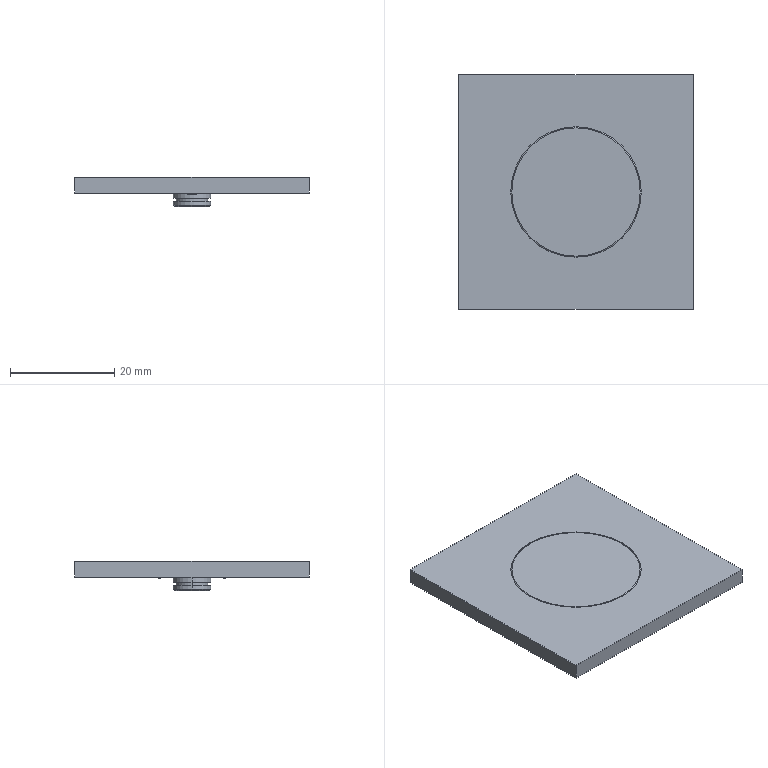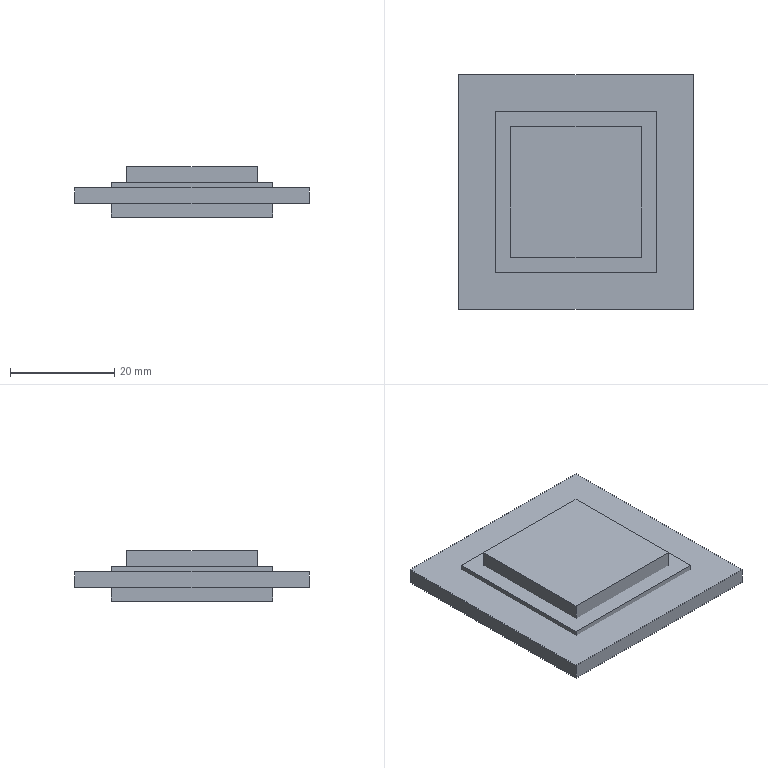CAM job | NX | 3-axis milling | part box 45 x 45 x 5.6 mm | stock box 45 x 45 x 9.6 mm
Tools:
number,name,description,diameter,corner_radius,flute_length,length,flutes
1,D6A45,Milling Tool-5 Parameters,6.0,0.0,50.0,75.0,2
14,D10JING,Milling Tool-5 Parameters,10.0,0.0,50.0,75.0,2
17,D4,Milling Tool-5 Parameters,4.0,0.0,50.0,75.0,2
18,D2,Milling Tool-5 Parameters,2.0,0.0,50.0,75.0,2
12,D2R0.5,Milling Tool-5 Parameters,2.0,0.5,50.0,75.0,2
24,T8H0.6,Milling Tool-T Cutter,8.0,,0.6,25.0,4
Operations:
program,operation,operation_type,tool,method,geometry_group,spindle_rpm,surface_speed,feed_per_tooth,feed_cut,feed_plunge,cut_length_mm,path_length_mm,cut_time_min,machine_time_min
1,FLOOR_WALL,VolumeBased25DMillingOperation,D10JING,METHOD,A,9500.0,298.0,0.0658,1250.0,100.0,325.997,379.997,0.2608,0.2662
1,PLANAR_MILL,PlanarMilling,D6A45,METHOD,A,9500.0,179.0,0.0658,1250.0,100.0,90.155,149.155,0.0721,0.078
1,ZLEVEL_PROFILE,ZLevelMilling,D10JING,METHOD,A,9500.0,298.0,0.1316,2500.0,100.0,765.005,827.605,0.306,0.3123
1,ZLEVEL_PROFILE_COPY_1,ZLevelMilling,D10JING,METHOD,A,9500.0,298.0,0.0632,1200.0,100.0,118.345,186.545,0.0986,0.1054
2,FLOOR_WALL_COPY,VolumeBased25DMillingOperation,D10JING,METHOD,B,9500.0,298.0,0.0658,1250.0,100.0,971.988,1238.98,0.7776,0.8043
2,CAVITY_MILL,CavityMilling,D4,METHOD,B,9500.0,298.0,0.1579,3000.0,1000.0,1582.4,1735.748,0.5437,0.5591
2,FLOOR_WALL_1,VolumeBased25DMillingOperation,D4,METHOD,B,9500.0,298.0,0.0658,1250.0,100.0,406.058,624.819,0.3248,0.3467
2,CAVITY_MILL_COPY,CavityMilling,D2,METHOD,B,9500.0,59.0,0.0632,1200.0,1000.0,110.12,254.186,0.0948,0.1092
2,PLANAR_MILL_COPY,PlanarMilling,D6A45,METHOD,B,9500.0,179.0,0.0658,1250.0,100.0,33.426,92.426,0.0267,0.0326
2,PLANAR_MILL_COPY_COPY,PlanarMilling,D6A45,METHOD,B,9500.0,179.0,0.0658,1250.0,100.0,89.526,155.526,0.0716,0.0782
2,ZLEVEL_PROFILE_COPY_2,ZLevelMilling,D2R0.5,METHOD,B,9500.0,119.0,0.1316,2500.0,100.0,447.709,581.849,0.1791,0.1925
2,PLANAR_MILL_COPY_COPY_COPY,PlanarMilling,T8H0.6,METHOD,B,7000.0,175.0,0.0536,1500.0,100.0,98.383,161.583,0.0656,0.0719
PROGRAM,HOLE_MILLING,CylinderMilling,D10JING,METHOD,C,9500.0,298.0,0.1053,2000.0,100.0,311.698,371.698,0.1558,0.1618
PROGRAM,ZLEVEL_PROFILE_COPY_1_COPY_1,ZLevelMilling,D10JING,METHOD,C,9500.0,298.0,0.0632,1200.0,100.0,56.495,119.495,0.0471,0.0534